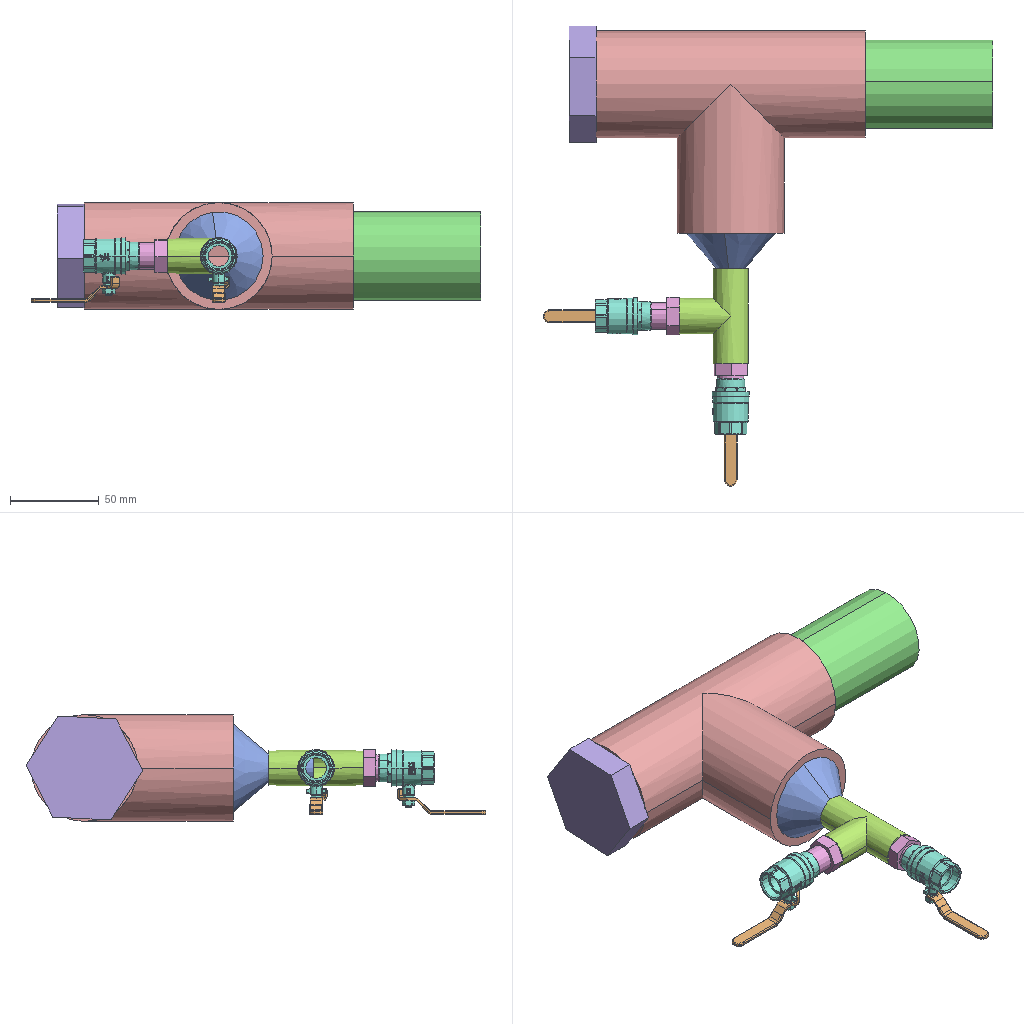Assembly | SolidWorks | 7 different items | 9 placed | box 253 x 259 x 60 mm
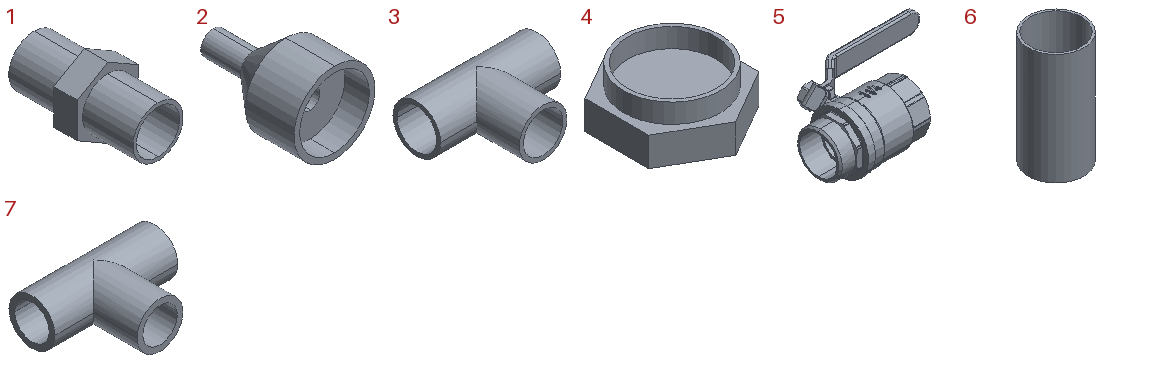Parts list (item | quantity | size | volume | features):
1 | x2 | 18.246 x 37 x 21.069 mm | 2425 mm3 | features ICE 3, Extrusion 1
2 | x1 | 50 x 75 x 50 mm | 53467 mm3 | features ICE 3, Chamfer 1, Extrusion 1
3 | x1 | 152 x 114.15 x 60.3 mm | 179160 mm3 | features ICE 2, Sweep 2
4 | x1 | 57.073 x 65.902 x 25 mm | 45330 mm3 | features Extrusion 1, ICE 1
5 | x2 | 60.8 x 36.67 x 20.9 mm | 5725 mm3 | features BaseBody 2, Scale 1
6 | x1 | 50 x 50 x 100 mm | 30159 mm3 | features Extrusion 1
7 | x1 | 53.5 x 39 x 20 mm | 9797 mm3 | features ICE 2, Sweep 2
Mates (type | each side: item.copy, entity, surface, feature):
Concentric | 3.1 face cylinder Sweep-thin part 2 | 2.1 face cylinder Boss-Extrude1
Coincident | 3.1 edge | 2.1 edge
Concentric | 2.1 face cylinder Boss-Extrude2 | 7.1 face cylinder Sweep-thin part 1
Concentric | 7.1 face cylinder Sweep-thin part 2 | 1.1 face cylinder Boss-Extrude3
Coincident | 7.1 face plane Sweep-thin part 2 | 1.1 face plane Boss-Extrude2
Coincident | 2.1 edge | 7.1 face plane Sweep-thin part 1
Concentric | 7.1 face cylinder Sweep-thin part 1 | 1.2 face cylinder Boss-Extrude3
Coincident | 7.1 face plane Sweep-thin part 1 | 1.2 face plane Boss-Extrude2
Concentric | 1.1 face cylinder Boss-Extrude1 | 5.1 face cylinder Base body G 1 1-4 _Default-1-solid1
Parallel | 5.1 face plane Base body G1 1-4_Default-1-solid1 | assembly plane
Concentric | 1.2 face cylinder Boss-Extrude1 | 5.2 face cylinder Base body G 1 1-4 _Default-1-solid1
Coincident | 5.1 face plane Base body G1 1-4_Default-1-solid1 | 5.2 face plane Base body G1 1-4_Default-1-solid1
Concentric | 3.1 face cylinder Sweep-thin part 1 | 4.1 face cylinder Boss-Extrude1
Coincident | 3.1 face plane Sweep-thin part 1 | 4.1 face plane Boss-Extrude2
Concentric | 3.1 face cylinder Sweep-thin part 1 | 6.1 face cylinder Boss-Extrude1